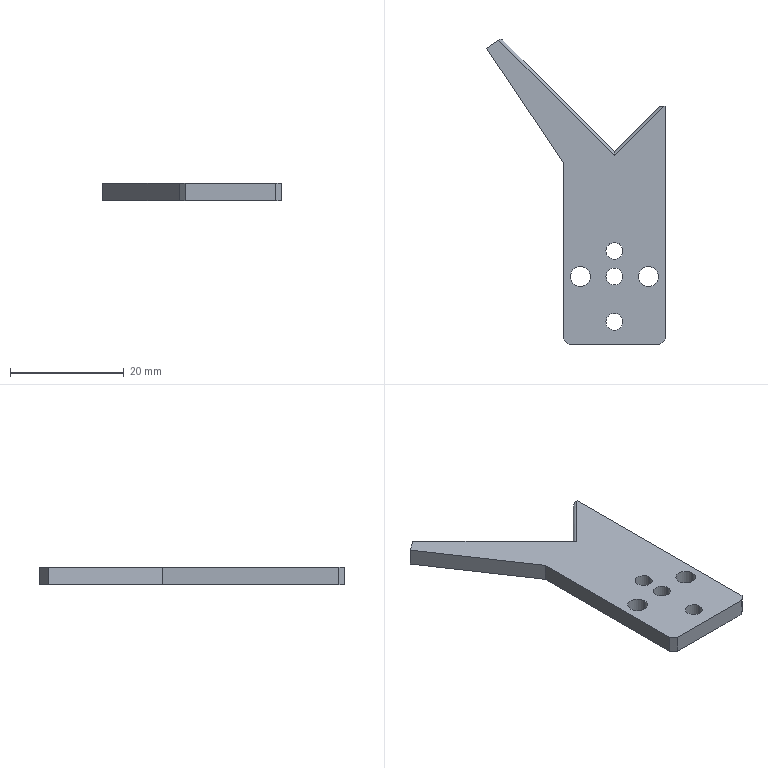Part | STEP file | 11-FG-E01711 | 1 solid | 28 faces | box 31.54 x 53.795 x 3 mm | volume 2242 mm3 | cylinder 16 | plane 12 | commonest cylinder face diameters 1 x6 3 x6 3.5 x4
STEP:
#1=CARTESIAN_POINT('',(1.5,-9.5,0.));
#2=VERTEX_POINT('',#1);
#3=CARTESIAN_POINT('',(-1.5,-9.5,0.));
#4=VERTEX_POINT('',#3);
#5=CARTESIAN_POINT('',(0.,-9.5,0.));
#6=DIRECTION('',(0.,0.,-1.));
#7=DIRECTION('',(-1.,0.,0.));
#8=AXIS2_PLACEMENT_3D('',#5,#6,#7);
#9=CIRCLE('',#8,1.5);
#10=EDGE_CURVE('',#2,#4,#9,.T.);
#11=ORIENTED_EDGE('',*,*,#10,.T.);
#12=CARTESIAN_POINT('',(-1.5,-9.5,3.));
#13=VERTEX_POINT('',#12);
#14=CARTESIAN_POINT('',(-1.5,-9.5,3.));
#15=DIRECTION('',(0.,0.,1.));
#16=VECTOR('',#15,1000.);
#17=LINE('',#14,#16);
#18=EDGE_CURVE('',#4,#13,#17,.T.);
#19=ORIENTED_EDGE('',*,*,#18,.T.);
#20=CARTESIAN_POINT('',(1.5,-9.5,3.));
#21=VERTEX_POINT('',#20);
#22=CARTESIAN_POINT('',(0.,-9.5,3.));
#23=DIRECTION('',(0.,0.,1.));
#24=DIRECTION('',(1.,0.,0.));
#25=AXIS2_PLACEMENT_3D('',#22,#23,#24);
#26=CIRCLE('',#25,1.5);
#27=EDGE_CURVE('',#13,#21,#26,.T.);
#28=ORIENTED_EDGE('',*,*,#27,.T.);
#29=CARTESIAN_POINT('',(1.5,-9.5,3.));
#30=DIRECTION('',(0.,0.,1.));
#31=VECTOR('',#30,1000.);
#32=LINE('',#29,#31);
#33=EDGE_CURVE('',#2,#21,#32,.T.);
#34=ORIENTED_EDGE('',*,*,#33,.F.);
#35=EDGE_LOOP('',(#11,#19,#28,#34));
#36=FACE_OUTER_BOUND('',#35,.T.);
#37=CARTESIAN_POINT('',(0.,-9.5,3.));
#38=DIRECTION('',(0.,0.,1.));
#39=DIRECTION('',(1.,0.,0.));
#40=AXIS2_PLACEMENT_3D('',#37,#38,#39);
#41=CYLINDRICAL_SURFACE('',#40,1.5);
#42=ADVANCED_FACE('',(#36),#41,.F.);
#43=CARTESIAN_POINT('',(1.5,-17.5,0.));
#44=VERTEX_POINT('',#43);
#45=CARTESIAN_POINT('',(-1.5,-17.5,0.));
#46=VERTEX_POINT('',#45);
#47=CARTESIAN_POINT('',(0.,-17.5,0.));
#48=DIRECTION('',(0.,0.,-1.));
#49=DIRECTION('',(-1.,0.,0.));
#50=AXIS2_PLACEMENT_3D('',#47,#48,#49);
#51=CIRCLE('',#50,1.5);
#52=EDGE_CURVE('',#44,#46,#51,.T.);
#53=ORIENTED_EDGE('',*,*,#52,.T.);
#54=CARTESIAN_POINT('',(-1.5,-17.5,3.));
#55=VERTEX_POINT('',#54);
#56=CARTESIAN_POINT('',(-1.5,-17.5,3.));
#57=DIRECTION('',(0.,0.,1.));
#58=VECTOR('',#57,1000.);
#59=LINE('',#56,#58);
#60=EDGE_CURVE('',#46,#55,#59,.T.);
#61=ORIENTED_EDGE('',*,*,#60,.T.);
#62=CARTESIAN_POINT('',(1.5,-17.5,3.));
#63=VERTEX_POINT('',#62);
#64=CARTESIAN_POINT('',(0.,-17.5,3.));
#65=DIRECTION('',(0.,0.,1.));
#66=DIRECTION('',(1.,0.,0.));
#67=AXIS2_PLACEMENT_3D('',#64,#65,#66);
#68=CIRCLE('',#67,1.5);
#69=EDGE_CURVE('',#55,#63,#68,.T.);
#70=ORIENTED_EDGE('',*,*,#69,.T.);
#71=CARTESIAN_POINT('',(1.5,-17.5,3.));
#72=DIRECTION('',(0.,0.,1.));
#73=VECTOR('',#72,1000.);
#74=LINE('',#71,#73);
#75=EDGE_CURVE('',#44,#63,#74,.T.);
#76=ORIENTED_EDGE('',*,*,#75,.F.);
#77=EDGE_LOOP('',(#53,#61,#70,#76));
#78=FACE_OUTER_BOUND('',#77,.T.);
#79=CARTESIAN_POINT('',(0.,-17.5,3.));
#80=DIRECTION('',(0.,0.,1.));
#81=DIRECTION('',(1.,0.,0.));
#82=AXIS2_PLACEMENT_3D('',#79,#80,#81);
#83=CYLINDRICAL_SURFACE('',#82,1.5);
#84=ADVANCED_FACE('',(#78),#83,.F.);
#85=CARTESIAN_POINT('',(1.5,-5.,0.));
#86=VERTEX_POINT('',#85);
#87=CARTESIAN_POINT('',(-1.5,-5.,0.));
#88=VERTEX_POINT('',#87);
#89=CARTESIAN_POINT('',(0.,-5.,0.));
#90=DIRECTION('',(0.,0.,-1.));
#91=DIRECTION('',(-1.,0.,0.));
#92=AXIS2_PLACEMENT_3D('',#89,#90,#91);
#93=CIRCLE('',#92,1.5);
#94=EDGE_CURVE('',#86,#88,#93,.T.);
#95=ORIENTED_EDGE('',*,*,#94,.T.);
#96=CARTESIAN_POINT('',(-1.5,-5.,3.));
#97=VERTEX_POINT('',#96);
#98=CARTESIAN_POINT('',(-1.5,-5.,3.));
#99=DIRECTION('',(0.,0.,1.));
#100=VECTOR('',#99,1000.);
#101=LINE('',#98,#100);
#102=EDGE_CURVE('',#88,#97,#101,.T.);
#103=ORIENTED_EDGE('',*,*,#102,.T.);
#104=CARTESIAN_POINT('',(1.5,-5.,3.));
#105=VERTEX_POINT('',#104);
#106=CARTESIAN_POINT('',(0.,-5.,3.));
#107=DIRECTION('',(0.,0.,1.));
#108=DIRECTION('',(1.,0.,0.));
#109=AXIS2_PLACEMENT_3D('',#106,#107,#108);
#110=CIRCLE('',#109,1.5);
#111=EDGE_CURVE('',#97,#105,#110,.T.);
#112=ORIENTED_EDGE('',*,*,#111,.T.);
#113=CARTESIAN_POINT('',(1.5,-5.,3.));
#114=DIRECTION('',(0.,0.,1.));
#115=VECTOR('',#114,1000.);
#116=LINE('',#113,#115);
#117=EDGE_CURVE('',#86,#105,#116,.T.);
#118=ORIENTED_EDGE('',*,*,#117,.F.);
#119=EDGE_LOOP('',(#95,#103,#112,#118));
#120=FACE_OUTER_BOUND('',#119,.T.);
#121=CARTESIAN_POINT('',(0.,-5.,3.));
#122=DIRECTION('',(0.,0.,1.));
#123=DIRECTION('',(1.,0.,0.));
#124=AXIS2_PLACEMENT_3D('',#121,#122,#123);
#125=CYLINDRICAL_SURFACE('',#124,1.5);
#126=ADVANCED_FACE('',(#120),#125,.F.);
#127=CARTESIAN_POINT('',(4.25,-9.5,0.));
#128=VERTEX_POINT('',#127);
#129=CARTESIAN_POINT('',(7.75,-9.5,0.));
#130=VERTEX_POINT('',#129);
#131=CARTESIAN_POINT('',(6.,-9.5,0.));
#132=DIRECTION('',(0.,0.,1.));
#133=DIRECTION('',(1.,0.,0.));
#134=AXIS2_PLACEMENT_3D('',#131,#132,#133);
#135=CIRCLE('',#134,1.75);
#136=EDGE_CURVE('',#128,#130,#135,.T.);
#137=ORIENTED_EDGE('',*,*,#136,.F.);
#138=CARTESIAN_POINT('',(4.25,-9.5,3.));
#139=VERTEX_POINT('',#138);
#140=CARTESIAN_POINT('',(4.25,-9.5,3.));
#141=DIRECTION('',(0.,0.,1.));
#142=VECTOR('',#141,1000.);
#143=LINE('',#140,#142);
#144=EDGE_CURVE('',#128,#139,#143,.T.);
#145=ORIENTED_EDGE('',*,*,#144,.T.);
#146=CARTESIAN_POINT('',(7.75,-9.5,3.));
#147=VERTEX_POINT('',#146);
#148=CARTESIAN_POINT('',(6.,-9.5,3.));
#149=DIRECTION('',(0.,0.,1.));
#150=DIRECTION('',(1.,0.,0.));
#151=AXIS2_PLACEMENT_3D('',#148,#149,#150);
#152=CIRCLE('',#151,1.75);
#153=EDGE_CURVE('',#139,#147,#152,.T.);
#154=ORIENTED_EDGE('',*,*,#153,.T.);
#155=CARTESIAN_POINT('',(7.75,-9.5,3.));
#156=DIRECTION('',(0.,0.,1.));
#157=VECTOR('',#156,1000.);
#158=LINE('',#155,#157);
#159=EDGE_CURVE('',#130,#147,#158,.T.);
#160=ORIENTED_EDGE('',*,*,#159,.F.);
#161=EDGE_LOOP('',(#137,#145,#154,#160));
#162=FACE_OUTER_BOUND('',#161,.T.);
#163=CARTESIAN_POINT('',(6.,-9.5,3.));
#164=DIRECTION('',(0.,0.,1.));
#165=DIRECTION('',(1.,0.,0.));
#166=AXIS2_PLACEMENT_3D('',#163,#164,#165);
#167=CYLINDRICAL_SURFACE('',#166,1.75);
#168=ADVANCED_FACE('',(#162),#167,.F.);
#169=CARTESIAN_POINT('',(-7.75,-9.5,0.));
#170=VERTEX_POINT('',#169);
#171=CARTESIAN_POINT('',(-4.25,-9.5,0.));
#172=VERTEX_POINT('',#171);
#173=CARTESIAN_POINT('',(-6.,-9.5,0.));
#174=DIRECTION('',(0.,0.,1.));
#175=DIRECTION('',(1.,0.,0.));
#176=AXIS2_PLACEMENT_3D('',#173,#174,#175);
#177=CIRCLE('',#176,1.75);
#178=EDGE_CURVE('',#170,#172,#177,.T.);
#179=ORIENTED_EDGE('',*,*,#178,.F.);
#180=CARTESIAN_POINT('',(-7.75,-9.5,3.));
#181=VERTEX_POINT('',#180);
#182=CARTESIAN_POINT('',(-7.75,-9.5,3.));
#183=DIRECTION('',(0.,0.,1.));
#184=VECTOR('',#183,1000.);
#185=LINE('',#182,#184);
#186=EDGE_CURVE('',#170,#181,#185,.T.);
#187=ORIENTED_EDGE('',*,*,#186,.T.);
#188=CARTESIAN_POINT('',(-4.25,-9.5,3.));
#189=VERTEX_POINT('',#188);
#190=CARTESIAN_POINT('',(-6.,-9.5,3.));
#191=DIRECTION('',(0.,0.,1.));
#192=DIRECTION('',(1.,0.,0.));
#193=AXIS2_PLACEMENT_3D('',#190,#191,#192);
#194=CIRCLE('',#193,1.75);
#195=EDGE_CURVE('',#181,#189,#194,.T.);
#196=ORIENTED_EDGE('',*,*,#195,.T.);
#197=CARTESIAN_POINT('',(-4.25,-9.5,3.));
#198=DIRECTION('',(0.,0.,1.));
#199=VECTOR('',#198,1000.);
#200=LINE('',#197,#199);
#201=EDGE_CURVE('',#172,#189,#200,.T.);
#202=ORIENTED_EDGE('',*,*,#201,.F.);
#203=EDGE_LOOP('',(#179,#187,#196,#202));
#204=FACE_OUTER_BOUND('',#203,.T.);
#205=CARTESIAN_POINT('',(-6.,-9.5,3.));
#206=DIRECTION('',(0.,0.,1.));
#207=DIRECTION('',(1.,0.,0.));
#208=AXIS2_PLACEMENT_3D('',#205,#206,#207);
#209=CYLINDRICAL_SURFACE('',#208,1.75);
#210=ADVANCED_FACE('',(#204),#209,.F.);
#211=CARTESIAN_POINT('',(-9.,10.555,0.));
#212=VERTEX_POINT('',#211);
#213=CARTESIAN_POINT('',(-9.,10.555,3.));
#214=VERTEX_POINT('',#213);
#215=CARTESIAN_POINT('',(-9.,10.555,-40.265));
#216=DIRECTION('',(0.,0.,1.));
#217=VECTOR('',#216,1000.);
#218=LINE('',#215,#217);
#219=EDGE_CURVE('',#212,#214,#218,.T.);
#220=ORIENTED_EDGE('',*,*,#219,.F.);
#221=CARTESIAN_POINT('',(-9.,-20.5,0.));
#222=VERTEX_POINT('',#221);
#223=CARTESIAN_POINT('',(-9.,-21.5,0.));
#224=DIRECTION('',(0.,-1.,0.));
#225=VECTOR('',#224,1000.);
#226=LINE('',#223,#225);
#227=EDGE_CURVE('',#212,#222,#226,.T.);
#228=ORIENTED_EDGE('',*,*,#227,.T.);
#229=CARTESIAN_POINT('',(-9.,-20.5,3.));
#230=VERTEX_POINT('',#229);
#231=CARTESIAN_POINT('',(-9.,-20.5,3.));
#232=DIRECTION('',(0.,0.,1.));
#233=VECTOR('',#232,1000.);
#234=LINE('',#231,#233);
#235=EDGE_CURVE('',#222,#230,#234,.T.);
#236=ORIENTED_EDGE('',*,*,#235,.T.);
#237=CARTESIAN_POINT('',(-9.,-21.5,3.));
#238=DIRECTION('',(0.,-1.,0.));
#239=VECTOR('',#238,1000.);
#240=LINE('',#237,#239);
#241=EDGE_CURVE('',#214,#230,#240,.T.);
#242=ORIENTED_EDGE('',*,*,#241,.F.);
#243=EDGE_LOOP('',(#220,#228,#236,#242));
#244=FACE_OUTER_BOUND('',#243,.T.);
#245=CARTESIAN_POINT('',(-9.,-21.5,3.));
#246=DIRECTION('',(1.,0.,0.));
#247=DIRECTION('',(0.,0.,-1.));
#248=AXIS2_PLACEMENT_3D('',#245,#246,#247);
#249=PLANE('',#248);
#250=ADVANCED_FACE('',(#244),#249,.F.);
#251=CARTESIAN_POINT('',(9.,-20.5,3.));
#252=VERTEX_POINT('',#251);
#253=CARTESIAN_POINT('',(9.,20.5,3.));
#254=VERTEX_POINT('',#253);
#255=CARTESIAN_POINT('',(9.,-21.5,3.));
#256=DIRECTION('',(0.,1.,0.));
#257=VECTOR('',#256,1000.);
#258=LINE('',#255,#257);
#259=EDGE_CURVE('',#252,#254,#258,.T.);
#260=ORIENTED_EDGE('',*,*,#259,.F.);
#261=CARTESIAN_POINT('',(9.,-20.5,0.));
#262=VERTEX_POINT('',#261);
#263=CARTESIAN_POINT('',(9.,-20.5,3.));
#264=DIRECTION('',(0.,0.,-1.));
#265=VECTOR('',#264,1000.);
#266=LINE('',#263,#265);
#267=EDGE_CURVE('',#252,#262,#266,.T.);
#268=ORIENTED_EDGE('',*,*,#267,.T.);
#269=CARTESIAN_POINT('',(9.,20.5,0.));
#270=VERTEX_POINT('',#269);
#271=CARTESIAN_POINT('',(9.,-21.5,0.));
#272=DIRECTION('',(0.,1.,0.));
#273=VECTOR('',#272,1000.);
#274=LINE('',#271,#273);
#275=EDGE_CURVE('',#262,#270,#274,.T.);
#276=ORIENTED_EDGE('',*,*,#275,.T.);
#277=CARTESIAN_POINT('',(9.,20.5,-7.));
#278=DIRECTION('',(0.,0.,1.));
#279=VECTOR('',#278,1000.);
#280=LINE('',#277,#279);
#281=EDGE_CURVE('',#270,#254,#280,.T.);
#282=ORIENTED_EDGE('',*,*,#281,.T.);
#283=EDGE_LOOP('',(#260,#268,#276,#282));
#284=FACE_OUTER_BOUND('',#283,.T.);
#285=CARTESIAN_POINT('',(9.,-21.5,3.));
#286=DIRECTION('',(-1.,0.,0.));
#287=DIRECTION('',(0.,0.,1.));
#288=AXIS2_PLACEMENT_3D('',#285,#286,#287);
#289=PLANE('',#288);
#290=ADVANCED_FACE('',(#284),#289,.F.);
#291=CARTESIAN_POINT('',(-8.,-21.5,0.));
#292=VERTEX_POINT('',#291);
#293=CARTESIAN_POINT('',(8.,-21.5,0.));
#294=VERTEX_POINT('',#293);
#295=CARTESIAN_POINT('',(-9.,-21.5,0.));
#296=DIRECTION('',(1.,0.,0.));
#297=VECTOR('',#296,1000.);
#298=LINE('',#295,#297);
#299=EDGE_CURVE('',#292,#294,#298,.T.);
#300=ORIENTED_EDGE('',*,*,#299,.T.);
#301=CARTESIAN_POINT('',(8.,-21.5,3.));
#302=VERTEX_POINT('',#301);
#303=CARTESIAN_POINT('',(8.,-21.5,3.));
#304=DIRECTION('',(0.,0.,1.));
#305=VECTOR('',#304,1000.);
#306=LINE('',#303,#305);
#307=EDGE_CURVE('',#294,#302,#306,.T.);
#308=ORIENTED_EDGE('',*,*,#307,.T.);
#309=CARTESIAN_POINT('',(-8.,-21.5,3.));
#310=VERTEX_POINT('',#309);
#311=CARTESIAN_POINT('',(-9.,-21.5,3.));
#312=DIRECTION('',(1.,0.,0.));
#313=VECTOR('',#312,1000.);
#314=LINE('',#311,#313);
#315=EDGE_CURVE('',#310,#302,#314,.T.);
#316=ORIENTED_EDGE('',*,*,#315,.F.);
#317=CARTESIAN_POINT('',(-8.,-21.5,3.));
#318=DIRECTION('',(0.,0.,-1.));
#319=VECTOR('',#318,1000.);
#320=LINE('',#317,#319);
#321=EDGE_CURVE('',#310,#292,#320,.T.);
#322=ORIENTED_EDGE('',*,*,#321,.T.);
#323=EDGE_LOOP('',(#300,#308,#316,#322));
#324=FACE_OUTER_BOUND('',#323,.T.);
#325=CARTESIAN_POINT('',(-9.,-21.5,3.));
#326=DIRECTION('',(0.,1.,0.));
#327=DIRECTION('',(0.,0.,1.));
#328=AXIS2_PLACEMENT_3D('',#325,#326,#327);
#329=PLANE('',#328);
#330=ADVANCED_FACE('',(#324),#329,.F.);
#331=CARTESIAN_POINT('',(0.,-9.5,3.));
#332=DIRECTION('',(0.,0.,1.));
#333=DIRECTION('',(1.,0.,0.));
#334=AXIS2_PLACEMENT_3D('',#331,#332,#333);
#335=CIRCLE('',#334,1.5);
#336=EDGE_CURVE('',#21,#13,#335,.T.);
#337=ORIENTED_EDGE('',*,*,#336,.F.);
#338=ORIENTED_EDGE('',*,*,#27,.F.);
#339=EDGE_LOOP('',(#337,#338));
#340=FACE_BOUND('',#339,.T.);
#341=CARTESIAN_POINT('',(0.,-17.5,3.));
#342=DIRECTION('',(0.,0.,1.));
#343=DIRECTION('',(1.,0.,0.));
#344=AXIS2_PLACEMENT_3D('',#341,#342,#343);
#345=CIRCLE('',#344,1.5);
#346=EDGE_CURVE('',#63,#55,#345,.T.);
#347=ORIENTED_EDGE('',*,*,#346,.F.);
#348=ORIENTED_EDGE('',*,*,#69,.F.);
#349=EDGE_LOOP('',(#347,#348));
#350=FACE_BOUND('',#349,.T.);
#351=CARTESIAN_POINT('',(0.,-5.,3.));
#352=DIRECTION('',(0.,0.,1.));
#353=DIRECTION('',(1.,0.,0.));
#354=AXIS2_PLACEMENT_3D('',#351,#352,#353);
#355=CIRCLE('',#354,1.5);
#356=EDGE_CURVE('',#105,#97,#355,.T.);
#357=ORIENTED_EDGE('',*,*,#356,.F.);
#358=ORIENTED_EDGE('',*,*,#111,.F.);
#359=EDGE_LOOP('',(#357,#358));
#360=FACE_BOUND('',#359,.T.);
#361=CARTESIAN_POINT('',(6.,-9.5,3.));
#362=DIRECTION('',(0.,0.,1.));
#363=DIRECTION('',(1.,0.,0.));
#364=AXIS2_PLACEMENT_3D('',#361,#362,#363);
#365=CIRCLE('',#364,1.75);
#366=EDGE_CURVE('',#147,#139,#365,.T.);
#367=ORIENTED_EDGE('',*,*,#366,.F.);
#368=ORIENTED_EDGE('',*,*,#153,.F.);
#369=EDGE_LOOP('',(#367,#368));
#370=FACE_BOUND('',#369,.T.);
#371=CARTESIAN_POINT('',(-6.,-9.5,3.));
#372=DIRECTION('',(0.,0.,1.));
#373=DIRECTION('',(1.,0.,0.));
#374=AXIS2_PLACEMENT_3D('',#371,#372,#373);
#375=CIRCLE('',#374,1.75);
#376=EDGE_CURVE('',#189,#181,#375,.T.);
#377=ORIENTED_EDGE('',*,*,#376,.F.);
#378=ORIENTED_EDGE('',*,*,#195,.F.);
#379=EDGE_LOOP('',(#377,#378));
#380=FACE_BOUND('',#379,.T.);
#381=CARTESIAN_POINT('',(8.707,20.5,3.));
#382=VERTEX_POINT('',#381);
#383=CARTESIAN_POINT('',(0.,20.5,3.));
#384=DIRECTION('',(1.,0.,0.));
#385=VECTOR('',#384,1000.);
#386=LINE('',#383,#385);
#387=EDGE_CURVE('',#382,#254,#386,.T.);
#388=ORIENTED_EDGE('',*,*,#387,.F.);
#389=CARTESIAN_POINT('',(0.,11.793,3.));
#390=VERTEX_POINT('',#389);
#391=CARTESIAN_POINT('',(-5.896,5.896,3.));
#392=DIRECTION('',(-0.7071,-0.7071,0.));
#393=VECTOR('',#392,1000.);
#394=LINE('',#391,#393);
#395=EDGE_CURVE('',#382,#390,#394,.T.);
#396=ORIENTED_EDGE('',*,*,#395,.T.);
#397=CARTESIAN_POINT('',(-20.363,32.155,3.));
#398=VERTEX_POINT('',#397);
#399=CARTESIAN_POINT('',(5.896,5.896,3.));
#400=DIRECTION('',(-0.7071,0.7071,0.));
#401=VECTOR('',#400,1000.);
#402=LINE('',#399,#401);
#403=EDGE_CURVE('',#390,#398,#402,.T.);
#404=ORIENTED_EDGE('',*,*,#403,.T.);
#405=CARTESIAN_POINT('',(-22.54,30.691,3.));
#406=VERTEX_POINT('',#405);
#407=CARTESIAN_POINT('',(-22.54,30.691,3.));
#408=DIRECTION('',(0.8298,0.558,0.));
#409=VECTOR('',#408,1000.);
#410=LINE('',#407,#409);
#411=EDGE_CURVE('',#406,#398,#410,.T.);
#412=ORIENTED_EDGE('',*,*,#411,.F.);
#413=CARTESIAN_POINT('',(-31.468,43.968,3.));
#414=DIRECTION('',(0.558,-0.8298,0.));
#415=VECTOR('',#414,1000.);
#416=LINE('',#413,#415);
#417=EDGE_CURVE('',#406,#214,#416,.T.);
#418=ORIENTED_EDGE('',*,*,#417,.T.);
#419=ORIENTED_EDGE('',*,*,#241,.T.);
#420=CARTESIAN_POINT('',(-8.,-21.5,3.));
#421=DIRECTION('',(0.7071,-0.7071,0.));
#422=VECTOR('',#421,1000.);
#423=LINE('',#420,#422);
#424=EDGE_CURVE('',#230,#310,#423,.T.);
#425=ORIENTED_EDGE('',*,*,#424,.T.);
#426=ORIENTED_EDGE('',*,*,#315,.T.);
#427=CARTESIAN_POINT('',(9.,-20.5,3.));
#428=DIRECTION('',(0.7071,0.7071,0.));
#429=VECTOR('',#428,1000.);
#430=LINE('',#427,#429);
#431=EDGE_CURVE('',#302,#252,#430,.T.);
#432=ORIENTED_EDGE('',*,*,#431,.T.);
#433=ORIENTED_EDGE('',*,*,#259,.T.);
#434=EDGE_LOOP('',(#388,#396,#404,#412,#418,#419,#425,#426,#432,#433));
#435=FACE_OUTER_BOUND('',#434,.T.);
#436=CARTESIAN_POINT('',(0.,0.,3.));
#437=DIRECTION('',(0.,0.,-1.));
#438=DIRECTION('',(-1.,0.,0.));
#439=AXIS2_PLACEMENT_3D('',#436,#437,#438);
#440=PLANE('',#439);
#441=ADVANCED_FACE('',(#340,#350,#360,#370,#380,#435),#440,.F.);
#442=CARTESIAN_POINT('',(-20.363,32.155,0.));
#443=VERTEX_POINT('',#442);
#444=CARTESIAN_POINT('',(-22.54,30.691,0.));
#445=VERTEX_POINT('',#444);
#446=CARTESIAN_POINT('',(-21.23,31.572,0.));
#447=DIRECTION('',(-0.8298,-0.558,0.));
#448=VECTOR('',#447,1000.);
#449=LINE('',#446,#448);
#450=EDGE_CURVE('',#443,#445,#449,.T.);
#451=ORIENTED_EDGE('',*,*,#450,.F.);
#452=CARTESIAN_POINT('',(0.,11.793,0.));
#453=VERTEX_POINT('',#452);
#454=CARTESIAN_POINT('',(-0.3536,12.146,0.));
#455=DIRECTION('',(0.7071,-0.7071,0.));
#456=VECTOR('',#455,1000.);
#457=LINE('',#454,#456);
#458=EDGE_CURVE('',#443,#453,#457,.T.);
#459=ORIENTED_EDGE('',*,*,#458,.T.);
#460=CARTESIAN_POINT('',(8.707,20.5,0.));
#461=VERTEX_POINT('',#460);
#462=CARTESIAN_POINT('',(8.354,20.146,0.));
#463=DIRECTION('',(0.7071,0.7071,0.));
#464=VECTOR('',#463,1000.);
#465=LINE('',#462,#464);
#466=EDGE_CURVE('',#453,#461,#465,.T.);
#467=ORIENTED_EDGE('',*,*,#466,.T.);
#468=CARTESIAN_POINT('',(0.,20.5,0.));
#469=DIRECTION('',(-1.,0.,0.));
#470=VECTOR('',#469,1000.);
#471=LINE('',#468,#470);
#472=EDGE_CURVE('',#270,#461,#471,.T.);
#473=ORIENTED_EDGE('',*,*,#472,.F.);
#474=ORIENTED_EDGE('',*,*,#275,.F.);
#475=CARTESIAN_POINT('',(14.75,-14.75,0.));
#476=DIRECTION('',(-0.7071,-0.7071,0.));
#477=VECTOR('',#476,1000.);
#478=LINE('',#475,#477);
#479=EDGE_CURVE('',#262,#294,#478,.T.);
#480=ORIENTED_EDGE('',*,*,#479,.T.);
#481=ORIENTED_EDGE('',*,*,#299,.F.);
#482=CARTESIAN_POINT('',(-14.75,-14.75,0.));
#483=DIRECTION('',(-0.7071,0.7071,0.));
#484=VECTOR('',#483,1000.);
#485=LINE('',#482,#484);
#486=EDGE_CURVE('',#292,#222,#485,.T.);
#487=ORIENTED_EDGE('',*,*,#486,.T.);
#488=ORIENTED_EDGE('',*,*,#227,.F.);
#489=CARTESIAN_POINT('',(-31.468,43.968,0.));
#490=DIRECTION('',(0.558,-0.8298,0.));
#491=VECTOR('',#490,1000.);
#492=LINE('',#489,#491);
#493=EDGE_CURVE('',#445,#212,#492,.T.);
#494=ORIENTED_EDGE('',*,*,#493,.F.);
#495=EDGE_LOOP('',(#451,#459,#467,#473,#474,#480,#481,#487,#488,#494));
#496=FACE_OUTER_BOUND('',#495,.T.);
#497=ORIENTED_EDGE('',*,*,#10,.F.);
#498=CARTESIAN_POINT('',(0.,-9.5,0.));
#499=DIRECTION('',(0.,0.,-1.));
#500=DIRECTION('',(-1.,0.,0.));
#501=AXIS2_PLACEMENT_3D('',#498,#499,#500);
#502=CIRCLE('',#501,1.5);
#503=EDGE_CURVE('',#4,#2,#502,.T.);
#504=ORIENTED_EDGE('',*,*,#503,.F.);
#505=EDGE_LOOP('',(#497,#504));
#506=FACE_BOUND('',#505,.T.);
#507=ORIENTED_EDGE('',*,*,#52,.F.);
#508=CARTESIAN_POINT('',(0.,-17.5,0.));
#509=DIRECTION('',(0.,0.,-1.));
#510=DIRECTION('',(-1.,0.,0.));
#511=AXIS2_PLACEMENT_3D('',#508,#509,#510);
#512=CIRCLE('',#511,1.5);
#513=EDGE_CURVE('',#46,#44,#512,.T.);
#514=ORIENTED_EDGE('',*,*,#513,.F.);
#515=EDGE_LOOP('',(#507,#514));
#516=FACE_BOUND('',#515,.T.);
#517=ORIENTED_EDGE('',*,*,#94,.F.);
#518=CARTESIAN_POINT('',(0.,-5.,0.));
#519=DIRECTION('',(0.,0.,-1.));
#520=DIRECTION('',(-1.,0.,0.));
#521=AXIS2_PLACEMENT_3D('',#518,#519,#520);
#522=CIRCLE('',#521,1.5);
#523=EDGE_CURVE('',#88,#86,#522,.T.);
#524=ORIENTED_EDGE('',*,*,#523,.F.);
#525=EDGE_LOOP('',(#517,#524));
#526=FACE_BOUND('',#525,.T.);
#527=CARTESIAN_POINT('',(6.,-9.5,0.));
#528=DIRECTION('',(0.,0.,1.));
#529=DIRECTION('',(1.,0.,0.));
#530=AXIS2_PLACEMENT_3D('',#527,#528,#529);
#531=CIRCLE('',#530,1.75);
#532=EDGE_CURVE('',#130,#128,#531,.T.);
#533=ORIENTED_EDGE('',*,*,#532,.T.);
#534=ORIENTED_EDGE('',*,*,#136,.T.);
#535=EDGE_LOOP('',(#533,#534));
#536=FACE_BOUND('',#535,.T.);
#537=CARTESIAN_POINT('',(-6.,-9.5,0.));
#538=DIRECTION('',(0.,0.,1.));
#539=DIRECTION('',(1.,0.,0.));
#540=AXIS2_PLACEMENT_3D('',#537,#538,#539);
#541=CIRCLE('',#540,1.75);
#542=EDGE_CURVE('',#172,#170,#541,.T.);
#543=ORIENTED_EDGE('',*,*,#542,.T.);
#544=ORIENTED_EDGE('',*,*,#178,.T.);
#545=EDGE_LOOP('',(#543,#544));
#546=FACE_BOUND('',#545,.T.);
#547=CARTESIAN_POINT('',(0.,0.,0.));
#548=DIRECTION('',(0.,0.,-1.));
#549=DIRECTION('',(-1.,0.,0.));
#550=AXIS2_PLACEMENT_3D('',#547,#548,#549);
#551=PLANE('',#550);
#552=ADVANCED_FACE('',(#496,#506,#516,#526,#536,#546),#551,.T.);
#553=CARTESIAN_POINT('',(7.854,20.354,2.5));
#554=VERTEX_POINT('',#553);
#555=CARTESIAN_POINT('',(7.854,20.354,0.5));
#556=VERTEX_POINT('',#555);
#557=CARTESIAN_POINT('',(7.854,20.354,0.));
#558=DIRECTION('',(0.,0.,-1.));
#559=VECTOR('',#558,1000.);
#560=LINE('',#557,#559);
#561=EDGE_CURVE('',#554,#556,#560,.T.);
#562=ORIENTED_EDGE('',*,*,#561,.T.);
#563=CARTESIAN_POINT('',(0.,12.5,0.5));
#564=VERTEX_POINT('',#563);
#565=CARTESIAN_POINT('',(0.,12.5,0.5));
#566=DIRECTION('',(-0.7071,-0.7071,0.));
#567=VECTOR('',#566,1000.);
#568=LINE('',#565,#567);
#569=EDGE_CURVE('',#556,#564,#568,.T.);
#570=ORIENTED_EDGE('',*,*,#569,.T.);
#571=CARTESIAN_POINT('',(0.,12.5,2.5));
#572=VERTEX_POINT('',#571);
#573=CARTESIAN_POINT('',(0.,12.5,0.));
#574=DIRECTION('',(0.,0.,1.));
#575=VECTOR('',#574,1000.);
#576=LINE('',#573,#575);
#577=EDGE_CURVE('',#564,#572,#576,.T.);
#578=ORIENTED_EDGE('',*,*,#577,.T.);
#579=CARTESIAN_POINT('',(0.,12.5,2.5));
#580=DIRECTION('',(0.7071,0.7071,0.));
#581=VECTOR('',#580,1000.);
#582=LINE('',#579,#581);
#583=EDGE_CURVE('',#572,#554,#582,.T.);
#584=ORIENTED_EDGE('',*,*,#583,.T.);
#585=EDGE_LOOP('',(#562,#570,#578,#584));
#586=FACE_OUTER_BOUND('',#585,.T.);
#587=CARTESIAN_POINT('',(0.,12.5,0.));
#588=DIRECTION('',(0.7071,-0.7071,0.));
#589=DIRECTION('',(0.7071,0.7071,0.));
#590=AXIS2_PLACEMENT_3D('',#587,#588,#589);
#591=PLANE('',#590);
#592=ADVANCED_FACE('',(#586),#591,.F.);
#593=ORIENTED_EDGE('',*,*,#577,.F.);
#594=CARTESIAN_POINT('',(-19.649,32.149,0.5));
#595=VERTEX_POINT('',#594);
#596=CARTESIAN_POINT('',(-19.94,32.44,0.5));
#597=DIRECTION('',(-0.7071,0.7071,0.));
#598=VECTOR('',#597,1000.);
#599=LINE('',#596,#598);
#600=EDGE_CURVE('',#564,#595,#599,.T.);
#601=ORIENTED_EDGE('',*,*,#600,.T.);
#602=CARTESIAN_POINT('',(-19.649,32.149,2.5));
#603=VERTEX_POINT('',#602);
#604=CARTESIAN_POINT('',(-19.649,32.149,0.));
#605=DIRECTION('',(0.,0.,1.));
#606=VECTOR('',#605,1000.);
#607=LINE('',#604,#606);
#608=EDGE_CURVE('',#595,#603,#607,.T.);
#609=ORIENTED_EDGE('',*,*,#608,.T.);
#610=CARTESIAN_POINT('',(-9.,21.5,2.5));
#611=DIRECTION('',(0.7071,-0.7071,0.));
#612=VECTOR('',#611,1000.);
#613=LINE('',#610,#612);
#614=EDGE_CURVE('',#603,#572,#613,.T.);
#615=ORIENTED_EDGE('',*,*,#614,.T.);
#616=EDGE_LOOP('',(#593,#601,#609,#615));
#617=FACE_OUTER_BOUND('',#616,.T.);
#618=CARTESIAN_POINT('',(-9.,21.5,0.));
#619=DIRECTION('',(-0.7071,-0.7071,0.));
#620=DIRECTION('',(0.7071,-0.7071,0.));
#621=AXIS2_PLACEMENT_3D('',#618,#619,#620);
#622=PLANE('',#621);
#623=ADVANCED_FACE('',(#617),#622,.F.);
#624=ORIENTED_EDGE('',*,*,#186,.F.);
#625=ORIENTED_EDGE('',*,*,#542,.F.);
#626=ORIENTED_EDGE('',*,*,#201,.T.);
#627=ORIENTED_EDGE('',*,*,#376,.T.);
#628=EDGE_LOOP('',(#624,#625,#626,#627));
#629=FACE_OUTER_BOUND('',#628,.T.);
#630=CARTESIAN_POINT('',(-6.,-9.5,3.));
#631=DIRECTION('',(0.,0.,1.));
#632=DIRECTION('',(1.,0.,0.));
#633=AXIS2_PLACEMENT_3D('',#630,#631,#632);
#634=CYLINDRICAL_SURFACE('',#633,1.75);
#635=ADVANCED_FACE('',(#629),#634,.F.);
#636=ORIENTED_EDGE('',*,*,#144,.F.);
#637=ORIENTED_EDGE('',*,*,#532,.F.);
#638=ORIENTED_EDGE('',*,*,#159,.T.);
#639=ORIENTED_EDGE('',*,*,#366,.T.);
#640=EDGE_LOOP('',(#636,#637,#638,#639));
#641=FACE_OUTER_BOUND('',#640,.T.);
#642=CARTESIAN_POINT('',(6.,-9.5,3.));
#643=DIRECTION('',(0.,0.,1.));
#644=DIRECTION('',(1.,0.,0.));
#645=AXIS2_PLACEMENT_3D('',#642,#643,#644);
#646=CYLINDRICAL_SURFACE('',#645,1.75);
#647=ADVANCED_FACE('',(#641),#646,.F.);
#648=ORIENTED_EDGE('',*,*,#472,.T.);
#649=CARTESIAN_POINT('',(8.207,20.5,0.1464));
#650=VERTEX_POINT('',#649);
#651=CARTESIAN_POINT('',(8.707,20.5,0.));
#652=CARTESIAN_POINT('',(8.517,20.5,0.));
#653=CARTESIAN_POINT('',(8.341,20.5,0.05143));
#654=CARTESIAN_POINT('',(8.207,20.5,0.1464));
#655=(BOUNDED_CURVE()B_SPLINE_CURVE(3,(#651,#652,#653,#654),.UNSPECIFIED.,.F.,.F.)B_SPLINE_CURVE_WITH_KNOTS((4,4),(4.712,5.498),.UNSPECIFIED.)CURVE()GEOMETRIC_REPRESENTATION_ITEM()RATIONAL_B_SPLINE_CURVE((1.,0.9493,0.9493,1.))REPRESENTATION_ITEM(''));
#656=EDGE_CURVE('',#461,#650,#655,.T.);
#657=ORIENTED_EDGE('',*,*,#656,.T.);
#658=CARTESIAN_POINT('',(8.207,20.5,2.854));
#659=VERTEX_POINT('',#658);
#660=CARTESIAN_POINT('',(8.207,20.5,-7.));
#661=DIRECTION('',(0.,0.,1.));
#662=VECTOR('',#661,1000.);
#663=LINE('',#660,#662);
#664=EDGE_CURVE('',#650,#659,#663,.T.);
#665=ORIENTED_EDGE('',*,*,#664,.T.);
#666=CARTESIAN_POINT('',(8.207,20.5,2.854));
#667=CARTESIAN_POINT('',(8.341,20.5,2.949));
#668=CARTESIAN_POINT('',(8.517,20.5,3.));
#669=CARTESIAN_POINT('',(8.707,20.5,3.));
#670=(BOUNDED_CURVE()B_SPLINE_CURVE(3,(#666,#667,#668,#669),.UNSPECIFIED.,.F.,.F.)B_SPLINE_CURVE_WITH_KNOTS((4,4),(3.927,4.712),.UNSPECIFIED.)CURVE()GEOMETRIC_REPRESENTATION_ITEM()RATIONAL_B_SPLINE_CURVE((1.,0.9493,0.9493,1.))REPRESENTATION_ITEM(''));
#671=EDGE_CURVE('',#659,#382,#670,.T.);
#672=ORIENTED_EDGE('',*,*,#671,.T.);
#673=ORIENTED_EDGE('',*,*,#387,.T.);
#674=ORIENTED_EDGE('',*,*,#281,.F.);
#675=EDGE_LOOP('',(#648,#657,#665,#672,#673,#674));
#676=FACE_OUTER_BOUND('',#675,.T.);
#677=CARTESIAN_POINT('',(0.,20.5,-7.));
#678=DIRECTION('',(0.,-1.,0.));
#679=DIRECTION('',(0.,0.,-1.));
#680=AXIS2_PLACEMENT_3D('',#677,#678,#679);
#681=PLANE('',#680);
#682=ADVANCED_FACE('',(#676),#681,.F.);
#683=ORIENTED_EDGE('',*,*,#102,.F.);
#684=ORIENTED_EDGE('',*,*,#523,.T.);
#685=ORIENTED_EDGE('',*,*,#117,.T.);
#686=ORIENTED_EDGE('',*,*,#356,.T.);
#687=EDGE_LOOP('',(#683,#684,#685,#686));
#688=FACE_OUTER_BOUND('',#687,.T.);
#689=CARTESIAN_POINT('',(0.,-5.,3.));
#690=DIRECTION('',(0.,0.,1.));
#691=DIRECTION('',(1.,0.,0.));
#692=AXIS2_PLACEMENT_3D('',#689,#690,#691);
#693=CYLINDRICAL_SURFACE('',#692,1.5);
#694=ADVANCED_FACE('',(#688),#693,.F.);
#695=ORIENTED_EDGE('',*,*,#60,.F.);
#696=ORIENTED_EDGE('',*,*,#513,.T.);
#697=ORIENTED_EDGE('',*,*,#75,.T.);
#698=ORIENTED_EDGE('',*,*,#346,.T.);
#699=EDGE_LOOP('',(#695,#696,#697,#698));
#700=FACE_OUTER_BOUND('',#699,.T.);
#701=CARTESIAN_POINT('',(0.,-17.5,3.));
#702=DIRECTION('',(0.,0.,1.));
#703=DIRECTION('',(1.,0.,0.));
#704=AXIS2_PLACEMENT_3D('',#701,#702,#703);
#705=CYLINDRICAL_SURFACE('',#704,1.5);
#706=ADVANCED_FACE('',(#700),#705,.F.);
#707=ORIENTED_EDGE('',*,*,#18,.F.);
#708=ORIENTED_EDGE('',*,*,#503,.T.);
#709=ORIENTED_EDGE('',*,*,#33,.T.);
#710=ORIENTED_EDGE('',*,*,#336,.T.);
#711=EDGE_LOOP('',(#707,#708,#709,#710));
#712=FACE_OUTER_BOUND('',#711,.T.);
#713=CARTESIAN_POINT('',(0.,-9.5,3.));
#714=DIRECTION('',(0.,0.,1.));
#715=DIRECTION('',(1.,0.,0.));
#716=AXIS2_PLACEMENT_3D('',#713,#714,#715);
#717=CYLINDRICAL_SURFACE('',#716,1.5);
#718=ADVANCED_FACE('',(#712),#717,.F.);
#719=ORIENTED_EDGE('',*,*,#431,.F.);
#720=ORIENTED_EDGE('',*,*,#307,.F.);
#721=ORIENTED_EDGE('',*,*,#479,.F.);
#722=ORIENTED_EDGE('',*,*,#267,.F.);
#723=EDGE_LOOP('',(#719,#720,#721,#722));
#724=FACE_OUTER_BOUND('',#723,.T.);
#725=CARTESIAN_POINT('',(9.,-20.5,3.));
#726=DIRECTION('',(-0.7071,0.7071,0.));
#727=DIRECTION('',(0.,0.,-1.));
#728=AXIS2_PLACEMENT_3D('',#725,#726,#727);
#729=PLANE('',#728);
#730=ADVANCED_FACE('',(#724),#729,.F.);
#731=ORIENTED_EDGE('',*,*,#424,.F.);
#732=ORIENTED_EDGE('',*,*,#235,.F.);
#733=ORIENTED_EDGE('',*,*,#486,.F.);
#734=ORIENTED_EDGE('',*,*,#321,.F.);
#735=EDGE_LOOP('',(#731,#732,#733,#734));
#736=FACE_OUTER_BOUND('',#735,.T.);
#737=CARTESIAN_POINT('',(-8.,-21.5,3.));
#738=DIRECTION('',(0.7071,0.7071,0.));
#739=DIRECTION('',(0.,0.,-1.));
#740=AXIS2_PLACEMENT_3D('',#737,#738,#739);
#741=PLANE('',#740);
#742=ADVANCED_FACE('',(#736),#741,.F.);
#743=CARTESIAN_POINT('',(-22.54,30.691,-40.265));
#744=DIRECTION('',(0.,0.,1.));
#745=VECTOR('',#744,1000.);
#746=LINE('',#743,#745);
#747=EDGE_CURVE('',#445,#406,#746,.T.);
#748=ORIENTED_EDGE('',*,*,#747,.F.);
#749=ORIENTED_EDGE('',*,*,#493,.T.);
#750=ORIENTED_EDGE('',*,*,#219,.T.);
#751=ORIENTED_EDGE('',*,*,#417,.F.);
#752=EDGE_LOOP('',(#748,#749,#750,#751));
#753=FACE_OUTER_BOUND('',#752,.T.);
#754=CARTESIAN_POINT('',(-31.468,43.968,-40.265));
#755=DIRECTION('',(-0.8298,-0.558,0.));
#756=DIRECTION('',(0.558,-0.8298,0.));
#757=AXIS2_PLACEMENT_3D('',#754,#755,#756);
#758=PLANE('',#757);
#759=ADVANCED_FACE('',(#753),#758,.T.);
#760=CARTESIAN_POINT('',(-20.281,32.21,2.991));
#761=VERTEX_POINT('',#760);
#762=CARTESIAN_POINT('',(-20.281,32.21,0.009322));
#763=VERTEX_POINT('',#762);
#764=CARTESIAN_POINT('',(-20.281,32.21,-7.));
#765=DIRECTION('',(0.,0.,-1.));
#766=VECTOR('',#765,1000.);
#767=LINE('',#764,#766);
#768=EDGE_CURVE('',#761,#763,#767,.T.);
#769=ORIENTED_EDGE('',*,*,#768,.T.);
#770=CARTESIAN_POINT('',(-20.281,32.21,0.009322));
#771=CARTESIAN_POINT('',(-20.308,32.192,0.003117));
#772=CARTESIAN_POINT('',(-20.335,32.174,0.));
#773=CARTESIAN_POINT('',(-20.363,32.155,0.));
#774=(BOUNDED_CURVE()B_SPLINE_CURVE(3,(#770,#771,#772,#773),.UNSPECIFIED.,.F.,.F.)B_SPLINE_CURVE_WITH_KNOTS((4,4),(4.519,4.712),.UNSPECIFIED.)CURVE()GEOMETRIC_REPRESENTATION_ITEM()RATIONAL_B_SPLINE_CURVE((1.,0.9969,0.9969,1.))REPRESENTATION_ITEM(''));
#775=EDGE_CURVE('',#763,#443,#774,.T.);
#776=ORIENTED_EDGE('',*,*,#775,.T.);
#777=ORIENTED_EDGE('',*,*,#450,.T.);
#778=ORIENTED_EDGE('',*,*,#747,.T.);
#779=ORIENTED_EDGE('',*,*,#411,.T.);
#780=CARTESIAN_POINT('',(-20.363,32.155,3.));
#781=CARTESIAN_POINT('',(-20.335,32.174,3.));
#782=CARTESIAN_POINT('',(-20.308,32.192,2.997));
#783=CARTESIAN_POINT('',(-20.281,32.21,2.991));
#784=(BOUNDED_CURVE()B_SPLINE_CURVE(3,(#780,#781,#782,#783),.UNSPECIFIED.,.F.,.F.)B_SPLINE_CURVE_WITH_KNOTS((4,4),(4.712,4.906),.UNSPECIFIED.)CURVE()GEOMETRIC_REPRESENTATION_ITEM()RATIONAL_B_SPLINE_CURVE((1.,0.9969,0.9969,1.))REPRESENTATION_ITEM(''));
#785=EDGE_CURVE('',#398,#761,#784,.T.);
#786=ORIENTED_EDGE('',*,*,#785,.T.);
#787=EDGE_LOOP('',(#769,#776,#777,#778,#779,#786));
#788=FACE_OUTER_BOUND('',#787,.T.);
#789=CARTESIAN_POINT('',(-22.54,30.691,-7.));
#790=DIRECTION('',(0.558,-0.8298,0.));
#791=DIRECTION('',(0.8298,0.558,0.));
#792=AXIS2_PLACEMENT_3D('',#789,#790,#791);
#793=PLANE('',#792);
#794=ADVANCED_FACE('',(#788),#793,.F.);
#795=CARTESIAN_POINT('',(-20.281,32.21,0.009322));
#796=CARTESIAN_POINT('',(-20.074,32.35,0.05733));
#797=CARTESIAN_POINT('',(-19.825,32.325,0.2502));
#798=CARTESIAN_POINT('',(-19.649,32.149,0.5));
#799=(BOUNDED_CURVE()B_SPLINE_CURVE(3,(#795,#796,#797,#798),.UNSPECIFIED.,.F.,.F.)B_SPLINE_CURVE_WITH_KNOTS((4,4),(0.1934,1.571),.UNSPECIFIED.)CURVE()GEOMETRIC_REPRESENTATION_ITEM()RATIONAL_B_SPLINE_CURVE((1.,0.8481,0.8481,1.))REPRESENTATION_ITEM(''));
#800=EDGE_CURVE('',#763,#595,#799,.T.);
#801=ORIENTED_EDGE('',*,*,#800,.F.);
#802=ORIENTED_EDGE('',*,*,#768,.F.);
#803=CARTESIAN_POINT('',(-19.649,32.149,2.5));
#804=CARTESIAN_POINT('',(-19.825,32.325,2.75));
#805=CARTESIAN_POINT('',(-20.074,32.35,2.943));
#806=CARTESIAN_POINT('',(-20.281,32.21,2.991));
#807=(BOUNDED_CURVE()B_SPLINE_CURVE(3,(#803,#804,#805,#806),.UNSPECIFIED.,.F.,.F.)B_SPLINE_CURVE_WITH_KNOTS((4,4),(1.571,2.948),.UNSPECIFIED.)CURVE()GEOMETRIC_REPRESENTATION_ITEM()RATIONAL_B_SPLINE_CURVE((1.,0.8481,0.8481,1.))REPRESENTATION_ITEM(''));
#808=EDGE_CURVE('',#603,#761,#807,.T.);
#809=ORIENTED_EDGE('',*,*,#808,.F.);
#810=ORIENTED_EDGE('',*,*,#608,.F.);
#811=EDGE_LOOP('',(#801,#802,#809,#810));
#812=FACE_OUTER_BOUND('',#811,.T.);
#813=CARTESIAN_POINT('',(-20.002,31.795,0.));
#814=DIRECTION('',(0.,0.,1.));
#815=DIRECTION('',(1.,0.,0.));
#816=AXIS2_PLACEMENT_3D('',#813,#814,#815);
#817=CYLINDRICAL_SURFACE('',#816,0.5);
#818=ADVANCED_FACE('',(#812),#817,.T.);
#819=ORIENTED_EDGE('',*,*,#785,.F.);
#820=ORIENTED_EDGE('',*,*,#403,.F.);
#821=CARTESIAN_POINT('',(0.,12.5,2.5));
#822=CARTESIAN_POINT('',(0.,12.5,2.793));
#823=CARTESIAN_POINT('',(0.,12.207,3.));
#824=CARTESIAN_POINT('',(0.,11.793,3.));
#825=(BOUNDED_CURVE()B_SPLINE_CURVE(3,(#821,#822,#823,#824),.UNSPECIFIED.,.F.,.F.)B_SPLINE_CURVE_WITH_KNOTS((4,4),(0.,1.571),.UNSPECIFIED.)CURVE()GEOMETRIC_REPRESENTATION_ITEM()RATIONAL_B_SPLINE_CURVE((1.,0.8047,0.8047,1.))REPRESENTATION_ITEM(''));
#826=EDGE_CURVE('',#572,#390,#825,.T.);
#827=ORIENTED_EDGE('',*,*,#826,.F.);
#828=ORIENTED_EDGE('',*,*,#614,.F.);
#829=ORIENTED_EDGE('',*,*,#808,.T.);
#830=EDGE_LOOP('',(#819,#820,#827,#828,#829));
#831=FACE_OUTER_BOUND('',#830,.T.);
#832=CARTESIAN_POINT('',(-9.354,21.146,2.5));
#833=DIRECTION('',(0.7071,-0.7071,0.));
#834=DIRECTION('',(0.7071,0.7071,0.));
#835=AXIS2_PLACEMENT_3D('',#832,#833,#834);
#836=CYLINDRICAL_SURFACE('',#835,0.5);
#837=ADVANCED_FACE('',(#831),#836,.T.);
#838=ORIENTED_EDGE('',*,*,#800,.T.);
#839=ORIENTED_EDGE('',*,*,#600,.F.);
#840=CARTESIAN_POINT('',(0.,11.793,0.));
#841=CARTESIAN_POINT('',(0.,12.207,0.));
#842=CARTESIAN_POINT('',(0.,12.5,0.2071));
#843=CARTESIAN_POINT('',(0.,12.5,0.5));
#844=(BOUNDED_CURVE()B_SPLINE_CURVE(3,(#840,#841,#842,#843),.UNSPECIFIED.,.F.,.F.)B_SPLINE_CURVE_WITH_KNOTS((4,4),(4.712,6.283),.UNSPECIFIED.)CURVE()GEOMETRIC_REPRESENTATION_ITEM()RATIONAL_B_SPLINE_CURVE((1.,0.8047,0.8047,1.))REPRESENTATION_ITEM(''));
#845=EDGE_CURVE('',#453,#564,#844,.T.);
#846=ORIENTED_EDGE('',*,*,#845,.F.);
#847=ORIENTED_EDGE('',*,*,#458,.F.);
#848=ORIENTED_EDGE('',*,*,#775,.F.);
#849=EDGE_LOOP('',(#838,#839,#846,#847,#848));
#850=FACE_OUTER_BOUND('',#849,.T.);
#851=CARTESIAN_POINT('',(5.896,5.896,0.5));
#852=DIRECTION('',(-0.7071,0.7071,0.));
#853=DIRECTION('',(-0.7071,-0.7071,0.));
#854=AXIS2_PLACEMENT_3D('',#851,#852,#853);
#855=CYLINDRICAL_SURFACE('',#854,0.5);
#856=ADVANCED_FACE('',(#850),#855,.T.);
#857=ORIENTED_EDGE('',*,*,#395,.F.);
#858=ORIENTED_EDGE('',*,*,#671,.F.);
#859=CARTESIAN_POINT('',(7.854,20.354,2.5));
#860=CARTESIAN_POINT('',(7.949,20.449,2.634));
#861=CARTESIAN_POINT('',(8.073,20.5,2.759));
#862=CARTESIAN_POINT('',(8.207,20.5,2.854));
#863=(BOUNDED_CURVE()B_SPLINE_CURVE(3,(#859,#860,#861,#862),.UNSPECIFIED.,.F.,.F.)B_SPLINE_CURVE_WITH_KNOTS((4,4),(4.712,5.498),.UNSPECIFIED.)CURVE()GEOMETRIC_REPRESENTATION_ITEM()RATIONAL_B_SPLINE_CURVE((1.,0.9493,0.9493,1.))REPRESENTATION_ITEM(''));
#864=EDGE_CURVE('',#554,#659,#863,.T.);
#865=ORIENTED_EDGE('',*,*,#864,.F.);
#866=ORIENTED_EDGE('',*,*,#583,.F.);
#867=ORIENTED_EDGE('',*,*,#826,.T.);
#868=EDGE_LOOP('',(#857,#858,#865,#866,#867));
#869=FACE_OUTER_BOUND('',#868,.T.);
#870=CARTESIAN_POINT('',(0.3536,12.146,2.5));
#871=DIRECTION('',(0.7071,0.7071,0.));
#872=DIRECTION('',(-0.7071,0.7071,0.));
#873=AXIS2_PLACEMENT_3D('',#870,#871,#872);
#874=CYLINDRICAL_SURFACE('',#873,0.5);
#875=ADVANCED_FACE('',(#869),#874,.T.);
#876=ORIENTED_EDGE('',*,*,#845,.T.);
#877=ORIENTED_EDGE('',*,*,#569,.F.);
#878=CARTESIAN_POINT('',(8.207,20.5,0.1464));
#879=CARTESIAN_POINT('',(8.073,20.5,0.2415));
#880=CARTESIAN_POINT('',(7.949,20.449,0.3656));
#881=CARTESIAN_POINT('',(7.854,20.354,0.5));
#882=(BOUNDED_CURVE()B_SPLINE_CURVE(3,(#878,#879,#880,#881),.UNSPECIFIED.,.F.,.F.)B_SPLINE_CURVE_WITH_KNOTS((4,4),(3.927,4.712),.UNSPECIFIED.)CURVE()GEOMETRIC_REPRESENTATION_ITEM()RATIONAL_B_SPLINE_CURVE((1.,0.9493,0.9493,1.))REPRESENTATION_ITEM(''));
#883=EDGE_CURVE('',#650,#556,#882,.T.);
#884=ORIENTED_EDGE('',*,*,#883,.F.);
#885=ORIENTED_EDGE('',*,*,#656,.F.);
#886=ORIENTED_EDGE('',*,*,#466,.F.);
#887=EDGE_LOOP('',(#876,#877,#884,#885,#886));
#888=FACE_OUTER_BOUND('',#887,.T.);
#889=CARTESIAN_POINT('',(-5.896,5.896,0.5));
#890=DIRECTION('',(-0.7071,-0.7071,0.));
#891=DIRECTION('',(0.7071,-0.7071,0.));
#892=AXIS2_PLACEMENT_3D('',#889,#890,#891);
#893=CYLINDRICAL_SURFACE('',#892,0.5);
#894=ADVANCED_FACE('',(#888),#893,.T.);
#895=ORIENTED_EDGE('',*,*,#864,.T.);
#896=ORIENTED_EDGE('',*,*,#664,.F.);
#897=ORIENTED_EDGE('',*,*,#883,.T.);
#898=ORIENTED_EDGE('',*,*,#561,.F.);
#899=EDGE_LOOP('',(#895,#896,#897,#898));
#900=FACE_OUTER_BOUND('',#899,.T.);
#901=CARTESIAN_POINT('',(8.207,20.,0.));
#902=DIRECTION('',(0.,0.,-1.));
#903=DIRECTION('',(-1.,0.,0.));
#904=AXIS2_PLACEMENT_3D('',#901,#902,#903);
#905=CYLINDRICAL_SURFACE('',#904,0.5);
#906=ADVANCED_FACE('',(#900),#905,.T.);
#907=CLOSED_SHELL('',(#42,#84,#126,#168,#210,#250,#290,#330,#441,#552,#592,#623,#635,#647,#682,#694,#706,#718,#730,#742,#759,#794,#818,#837,#856,#875,#894,#906));
#908=MANIFOLD_SOLID_BREP('',#907);
#909=CARTESIAN_POINT('',(0.,0.,0.));
#910=DIRECTION('',(0.,0.,1.));
#911=DIRECTION('',(1.,0.,0.));
#912=AXIS2_PLACEMENT_3D('',#909,#910,#911);
#913=(LENGTH_UNIT()NAMED_UNIT(*)SI_UNIT(.MILLI.,.METRE.));
#914=UNCERTAINTY_MEASURE_WITH_UNIT(LENGTH_MEASURE(0.00001),#913,'','');
#915=(NAMED_UNIT(*)PLANE_ANGLE_UNIT()SI_UNIT($,.RADIAN.));
#916=(NAMED_UNIT(*)SI_UNIT($,.STERADIAN.)SOLID_ANGLE_UNIT());
#917=(GEOMETRIC_REPRESENTATION_CONTEXT(3)GLOBAL_UNCERTAINTY_ASSIGNED_CONTEXT((#914))GLOBAL_UNIT_ASSIGNED_CONTEXT((#913,#915,#916))REPRESENTATION_CONTEXT('',''));
#918=ADVANCED_BREP_SHAPE_REPRESENTATION('',(#908,#912),#917);